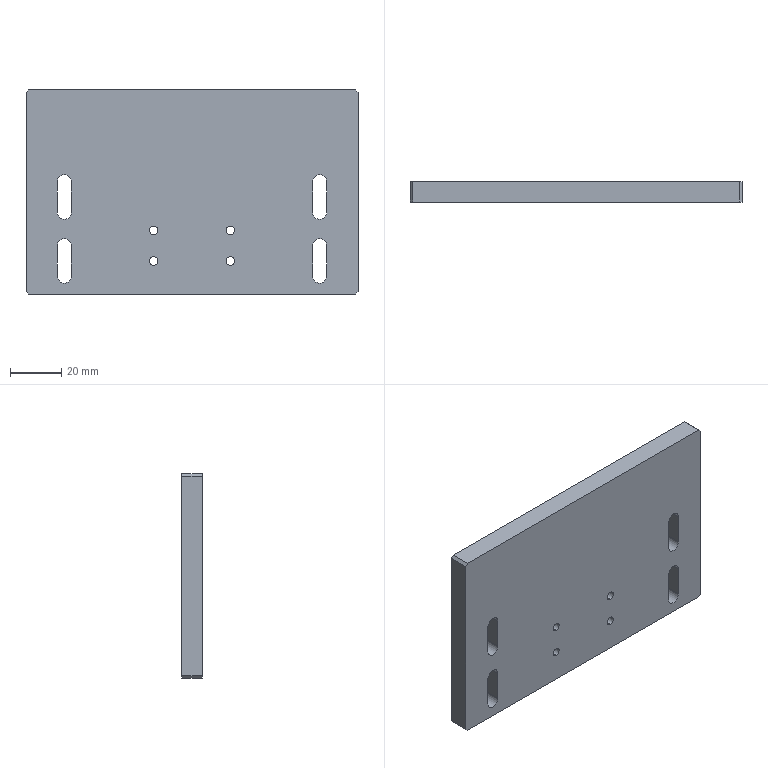Part | NX | features BREP 1 | 1 solid | 38 faces | box 130 x 8 x 80 mm | volume 80038 mm3 | cylinder 20 | plane 18 | commonest cylinder face diameters 5.5 x12 3.3 x8
STEP:
#1=CARTESIAN_POINT('',(15.,-4.,-16.65));
#2=VERTEX_POINT('',#1);
#3=CARTESIAN_POINT('',(15.,-4.,-13.35));
#4=VERTEX_POINT('',#3);
#5=CARTESIAN_POINT('',(15.,-4.,-15.));
#6=DIRECTION('',(0.,1.,0.));
#7=DIRECTION('',(0.,0.,1.));
#8=AXIS2_PLACEMENT_3D('',#5,#6,#7);
#9=CIRCLE('',#8,1.65);
#10=EDGE_CURVE('',#2,#4,#9,.T.);
#11=ORIENTED_EDGE('',*,*,#10,.F.);
#12=CARTESIAN_POINT('',(15.,4.,-16.65));
#13=VERTEX_POINT('',#12);
#14=CARTESIAN_POINT('',(15.,4.,-16.65));
#15=DIRECTION('',(0.,1.,0.));
#16=VECTOR('',#15,1000.);
#17=LINE('',#14,#16);
#18=EDGE_CURVE('',#13,#2,#17,.F.);
#19=ORIENTED_EDGE('',*,*,#18,.F.);
#20=CARTESIAN_POINT('',(15.,4.,-13.35));
#21=VERTEX_POINT('',#20);
#22=CARTESIAN_POINT('',(15.,4.,-15.));
#23=DIRECTION('',(0.,1.,0.));
#24=DIRECTION('',(0.,0.,1.));
#25=AXIS2_PLACEMENT_3D('',#22,#23,#24);
#26=CIRCLE('',#25,1.65);
#27=EDGE_CURVE('',#13,#21,#26,.T.);
#28=ORIENTED_EDGE('',*,*,#27,.T.);
#29=CARTESIAN_POINT('',(15.,4.,-13.35));
#30=DIRECTION('',(0.,1.,0.));
#31=VECTOR('',#30,1000.);
#32=LINE('',#29,#31);
#33=EDGE_CURVE('',#21,#4,#32,.F.);
#34=ORIENTED_EDGE('',*,*,#33,.T.);
#35=EDGE_LOOP('',(#11,#19,#28,#34));
#36=FACE_BOUND('',#35,.T.);
#37=CARTESIAN_POINT('',(15.,4.,-15.));
#38=DIRECTION('',(0.,1.,0.));
#39=DIRECTION('',(0.,0.,1.));
#40=AXIS2_PLACEMENT_3D('',#37,#38,#39);
#41=CYLINDRICAL_SURFACE('',#40,1.65);
#42=ADVANCED_FACE('',(#36),#41,.F.);
#43=CARTESIAN_POINT('',(15.,-4.,-28.65));
#44=VERTEX_POINT('',#43);
#45=CARTESIAN_POINT('',(15.,-4.,-25.35));
#46=VERTEX_POINT('',#45);
#47=CARTESIAN_POINT('',(15.,-4.,-27.));
#48=DIRECTION('',(0.,1.,0.));
#49=DIRECTION('',(0.,0.,1.));
#50=AXIS2_PLACEMENT_3D('',#47,#48,#49);
#51=CIRCLE('',#50,1.65);
#52=EDGE_CURVE('',#44,#46,#51,.T.);
#53=ORIENTED_EDGE('',*,*,#52,.F.);
#54=CARTESIAN_POINT('',(15.,4.,-28.65));
#55=VERTEX_POINT('',#54);
#56=CARTESIAN_POINT('',(15.,4.,-28.65));
#57=DIRECTION('',(0.,1.,0.));
#58=VECTOR('',#57,1000.);
#59=LINE('',#56,#58);
#60=EDGE_CURVE('',#55,#44,#59,.F.);
#61=ORIENTED_EDGE('',*,*,#60,.F.);
#62=CARTESIAN_POINT('',(15.,4.,-25.35));
#63=VERTEX_POINT('',#62);
#64=CARTESIAN_POINT('',(15.,4.,-27.));
#65=DIRECTION('',(0.,1.,0.));
#66=DIRECTION('',(0.,0.,1.));
#67=AXIS2_PLACEMENT_3D('',#64,#65,#66);
#68=CIRCLE('',#67,1.65);
#69=EDGE_CURVE('',#55,#63,#68,.T.);
#70=ORIENTED_EDGE('',*,*,#69,.T.);
#71=CARTESIAN_POINT('',(15.,4.,-25.35));
#72=DIRECTION('',(0.,1.,0.));
#73=VECTOR('',#72,1000.);
#74=LINE('',#71,#73);
#75=EDGE_CURVE('',#63,#46,#74,.F.);
#76=ORIENTED_EDGE('',*,*,#75,.T.);
#77=EDGE_LOOP('',(#53,#61,#70,#76));
#78=FACE_BOUND('',#77,.T.);
#79=CARTESIAN_POINT('',(15.,4.,-27.));
#80=DIRECTION('',(0.,1.,0.));
#81=DIRECTION('',(0.,0.,1.));
#82=AXIS2_PLACEMENT_3D('',#79,#80,#81);
#83=CYLINDRICAL_SURFACE('',#82,1.65);
#84=ADVANCED_FACE('',(#78),#83,.F.);
#85=CARTESIAN_POINT('',(-15.,-4.,-16.65));
#86=VERTEX_POINT('',#85);
#87=CARTESIAN_POINT('',(-15.,-4.,-13.35));
#88=VERTEX_POINT('',#87);
#89=CARTESIAN_POINT('',(-15.,-4.,-15.));
#90=DIRECTION('',(0.,1.,0.));
#91=DIRECTION('',(0.,0.,1.));
#92=AXIS2_PLACEMENT_3D('',#89,#90,#91);
#93=CIRCLE('',#92,1.65);
#94=EDGE_CURVE('',#86,#88,#93,.T.);
#95=ORIENTED_EDGE('',*,*,#94,.F.);
#96=CARTESIAN_POINT('',(-15.,4.,-16.65));
#97=VERTEX_POINT('',#96);
#98=CARTESIAN_POINT('',(-15.,4.,-16.65));
#99=DIRECTION('',(0.,1.,0.));
#100=VECTOR('',#99,1000.);
#101=LINE('',#98,#100);
#102=EDGE_CURVE('',#97,#86,#101,.F.);
#103=ORIENTED_EDGE('',*,*,#102,.F.);
#104=CARTESIAN_POINT('',(-15.,4.,-13.35));
#105=VERTEX_POINT('',#104);
#106=CARTESIAN_POINT('',(-15.,4.,-15.));
#107=DIRECTION('',(0.,1.,0.));
#108=DIRECTION('',(0.,0.,1.));
#109=AXIS2_PLACEMENT_3D('',#106,#107,#108);
#110=CIRCLE('',#109,1.65);
#111=EDGE_CURVE('',#97,#105,#110,.T.);
#112=ORIENTED_EDGE('',*,*,#111,.T.);
#113=CARTESIAN_POINT('',(-15.,4.,-13.35));
#114=DIRECTION('',(0.,1.,0.));
#115=VECTOR('',#114,1000.);
#116=LINE('',#113,#115);
#117=EDGE_CURVE('',#105,#88,#116,.F.);
#118=ORIENTED_EDGE('',*,*,#117,.T.);
#119=EDGE_LOOP('',(#95,#103,#112,#118));
#120=FACE_BOUND('',#119,.T.);
#121=CARTESIAN_POINT('',(-15.,4.,-15.));
#122=DIRECTION('',(0.,1.,0.));
#123=DIRECTION('',(0.,0.,1.));
#124=AXIS2_PLACEMENT_3D('',#121,#122,#123);
#125=CYLINDRICAL_SURFACE('',#124,1.65);
#126=ADVANCED_FACE('',(#120),#125,.F.);
#127=CARTESIAN_POINT('',(-15.,-4.,-28.65));
#128=VERTEX_POINT('',#127);
#129=CARTESIAN_POINT('',(-15.,-4.,-25.35));
#130=VERTEX_POINT('',#129);
#131=CARTESIAN_POINT('',(-15.,-4.,-27.));
#132=DIRECTION('',(0.,1.,0.));
#133=DIRECTION('',(0.,0.,1.));
#134=AXIS2_PLACEMENT_3D('',#131,#132,#133);
#135=CIRCLE('',#134,1.65);
#136=EDGE_CURVE('',#128,#130,#135,.T.);
#137=ORIENTED_EDGE('',*,*,#136,.F.);
#138=CARTESIAN_POINT('',(-15.,4.,-28.65));
#139=VERTEX_POINT('',#138);
#140=CARTESIAN_POINT('',(-15.,4.,-28.65));
#141=DIRECTION('',(0.,1.,0.));
#142=VECTOR('',#141,1000.);
#143=LINE('',#140,#142);
#144=EDGE_CURVE('',#139,#128,#143,.F.);
#145=ORIENTED_EDGE('',*,*,#144,.F.);
#146=CARTESIAN_POINT('',(-15.,4.,-25.35));
#147=VERTEX_POINT('',#146);
#148=CARTESIAN_POINT('',(-15.,4.,-27.));
#149=DIRECTION('',(0.,1.,0.));
#150=DIRECTION('',(0.,0.,1.));
#151=AXIS2_PLACEMENT_3D('',#148,#149,#150);
#152=CIRCLE('',#151,1.65);
#153=EDGE_CURVE('',#139,#147,#152,.T.);
#154=ORIENTED_EDGE('',*,*,#153,.T.);
#155=CARTESIAN_POINT('',(-15.,4.,-25.35));
#156=DIRECTION('',(0.,1.,0.));
#157=VECTOR('',#156,1000.);
#158=LINE('',#155,#157);
#159=EDGE_CURVE('',#147,#130,#158,.F.);
#160=ORIENTED_EDGE('',*,*,#159,.T.);
#161=EDGE_LOOP('',(#137,#145,#154,#160));
#162=FACE_BOUND('',#161,.T.);
#163=CARTESIAN_POINT('',(-15.,4.,-27.));
#164=DIRECTION('',(0.,1.,0.));
#165=DIRECTION('',(0.,0.,1.));
#166=AXIS2_PLACEMENT_3D('',#163,#164,#165);
#167=CYLINDRICAL_SURFACE('',#166,1.65);
#168=ADVANCED_FACE('',(#162),#167,.F.);
#169=CARTESIAN_POINT('',(52.75,-4.,4.));
#170=VERTEX_POINT('',#169);
#171=CARTESIAN_POINT('',(50.,-4.,6.75));
#172=VERTEX_POINT('',#171);
#173=CARTESIAN_POINT('',(50.,-4.,4.));
#174=DIRECTION('',(0.,-1.,0.));
#175=DIRECTION('',(0.,0.,1.));
#176=AXIS2_PLACEMENT_3D('',#173,#174,#175);
#177=CIRCLE('',#176,2.75);
#178=EDGE_CURVE('',#170,#172,#177,.T.);
#179=ORIENTED_EDGE('',*,*,#178,.T.);
#180=CARTESIAN_POINT('',(50.,4.,6.75));
#181=VERTEX_POINT('',#180);
#182=CARTESIAN_POINT('',(50.,-6.,6.75));
#183=DIRECTION('',(0.,1.,0.));
#184=VECTOR('',#183,1000.);
#185=LINE('',#182,#184);
#186=EDGE_CURVE('',#172,#181,#185,.T.);
#187=ORIENTED_EDGE('',*,*,#186,.T.);
#188=CARTESIAN_POINT('',(52.75,4.,4.));
#189=VERTEX_POINT('',#188);
#190=CARTESIAN_POINT('',(50.,4.,4.));
#191=DIRECTION('',(0.,-1.,0.));
#192=DIRECTION('',(0.,0.,1.));
#193=AXIS2_PLACEMENT_3D('',#190,#191,#192);
#194=CIRCLE('',#193,2.75);
#195=EDGE_CURVE('',#189,#181,#194,.T.);
#196=ORIENTED_EDGE('',*,*,#195,.F.);
#197=CARTESIAN_POINT('',(52.75,-6.,4.));
#198=DIRECTION('',(0.,1.,0.));
#199=VECTOR('',#198,1000.);
#200=LINE('',#197,#199);
#201=EDGE_CURVE('',#170,#189,#200,.T.);
#202=ORIENTED_EDGE('',*,*,#201,.F.);
#203=EDGE_LOOP('',(#179,#187,#196,#202));
#204=FACE_BOUND('',#203,.T.);
#205=CARTESIAN_POINT('',(50.,-6.,4.));
#206=DIRECTION('',(0.,1.,0.));
#207=DIRECTION('',(0.,0.,1.));
#208=AXIS2_PLACEMENT_3D('',#205,#206,#207);
#209=CYLINDRICAL_SURFACE('',#208,2.75);
#210=ADVANCED_FACE('',(#204),#209,.F.);
#211=CARTESIAN_POINT('',(52.75,-4.,-21.));
#212=VERTEX_POINT('',#211);
#213=CARTESIAN_POINT('',(50.,-4.,-18.25));
#214=VERTEX_POINT('',#213);
#215=CARTESIAN_POINT('',(50.,-4.,-21.));
#216=DIRECTION('',(0.,-1.,0.));
#217=DIRECTION('',(0.,0.,1.));
#218=AXIS2_PLACEMENT_3D('',#215,#216,#217);
#219=CIRCLE('',#218,2.75);
#220=EDGE_CURVE('',#212,#214,#219,.T.);
#221=ORIENTED_EDGE('',*,*,#220,.T.);
#222=CARTESIAN_POINT('',(50.,4.,-18.25));
#223=VERTEX_POINT('',#222);
#224=CARTESIAN_POINT('',(50.,-6.,-18.25));
#225=DIRECTION('',(0.,1.,0.));
#226=VECTOR('',#225,1000.);
#227=LINE('',#224,#226);
#228=EDGE_CURVE('',#214,#223,#227,.T.);
#229=ORIENTED_EDGE('',*,*,#228,.T.);
#230=CARTESIAN_POINT('',(52.75,4.,-21.));
#231=VERTEX_POINT('',#230);
#232=CARTESIAN_POINT('',(50.,4.,-21.));
#233=DIRECTION('',(0.,-1.,0.));
#234=DIRECTION('',(0.,0.,1.));
#235=AXIS2_PLACEMENT_3D('',#232,#233,#234);
#236=CIRCLE('',#235,2.75);
#237=EDGE_CURVE('',#231,#223,#236,.T.);
#238=ORIENTED_EDGE('',*,*,#237,.F.);
#239=CARTESIAN_POINT('',(52.75,-6.,-21.));
#240=DIRECTION('',(0.,1.,0.));
#241=VECTOR('',#240,1000.);
#242=LINE('',#239,#241);
#243=EDGE_CURVE('',#212,#231,#242,.T.);
#244=ORIENTED_EDGE('',*,*,#243,.F.);
#245=EDGE_LOOP('',(#221,#229,#238,#244));
#246=FACE_BOUND('',#245,.T.);
#247=CARTESIAN_POINT('',(50.,-6.,-21.));
#248=DIRECTION('',(0.,1.,0.));
#249=DIRECTION('',(0.,0.,1.));
#250=AXIS2_PLACEMENT_3D('',#247,#248,#249);
#251=CYLINDRICAL_SURFACE('',#250,2.75);
#252=ADVANCED_FACE('',(#246),#251,.F.);
#253=CARTESIAN_POINT('',(-50.,-4.,6.75));
#254=VERTEX_POINT('',#253);
#255=CARTESIAN_POINT('',(-47.25,-4.,4.));
#256=VERTEX_POINT('',#255);
#257=CARTESIAN_POINT('',(-50.,-4.,4.));
#258=DIRECTION('',(0.,1.,0.));
#259=DIRECTION('',(0.,0.,1.));
#260=AXIS2_PLACEMENT_3D('',#257,#258,#259);
#261=CIRCLE('',#260,2.75);
#262=EDGE_CURVE('',#254,#256,#261,.T.);
#263=ORIENTED_EDGE('',*,*,#262,.F.);
#264=CARTESIAN_POINT('',(-50.,4.,6.75));
#265=VERTEX_POINT('',#264);
#266=CARTESIAN_POINT('',(-50.,-6.,6.75));
#267=DIRECTION('',(0.,1.,0.));
#268=VECTOR('',#267,1000.);
#269=LINE('',#266,#268);
#270=EDGE_CURVE('',#254,#265,#269,.T.);
#271=ORIENTED_EDGE('',*,*,#270,.T.);
#272=CARTESIAN_POINT('',(-47.25,4.,4.));
#273=VERTEX_POINT('',#272);
#274=CARTESIAN_POINT('',(-50.,4.,4.));
#275=DIRECTION('',(0.,1.,0.));
#276=DIRECTION('',(0.,0.,1.));
#277=AXIS2_PLACEMENT_3D('',#274,#275,#276);
#278=CIRCLE('',#277,2.75);
#279=EDGE_CURVE('',#265,#273,#278,.T.);
#280=ORIENTED_EDGE('',*,*,#279,.T.);
#281=CARTESIAN_POINT('',(-47.25,-6.,4.));
#282=DIRECTION('',(0.,1.,0.));
#283=VECTOR('',#282,1000.);
#284=LINE('',#281,#283);
#285=EDGE_CURVE('',#256,#273,#284,.T.);
#286=ORIENTED_EDGE('',*,*,#285,.F.);
#287=EDGE_LOOP('',(#263,#271,#280,#286));
#288=FACE_BOUND('',#287,.T.);
#289=CARTESIAN_POINT('',(-50.,-6.,4.));
#290=DIRECTION('',(0.,1.,0.));
#291=DIRECTION('',(0.,0.,1.));
#292=AXIS2_PLACEMENT_3D('',#289,#290,#291);
#293=CYLINDRICAL_SURFACE('',#292,2.75);
#294=ADVANCED_FACE('',(#288),#293,.F.);
#295=CARTESIAN_POINT('',(-50.,-4.,-18.25));
#296=VERTEX_POINT('',#295);
#297=CARTESIAN_POINT('',(-47.25,-4.,-21.));
#298=VERTEX_POINT('',#297);
#299=CARTESIAN_POINT('',(-50.,-4.,-21.));
#300=DIRECTION('',(0.,1.,0.));
#301=DIRECTION('',(0.,0.,1.));
#302=AXIS2_PLACEMENT_3D('',#299,#300,#301);
#303=CIRCLE('',#302,2.75);
#304=EDGE_CURVE('',#296,#298,#303,.T.);
#305=ORIENTED_EDGE('',*,*,#304,.F.);
#306=CARTESIAN_POINT('',(-50.,4.,-18.25));
#307=VERTEX_POINT('',#306);
#308=CARTESIAN_POINT('',(-50.,-6.,-18.25));
#309=DIRECTION('',(0.,1.,0.));
#310=VECTOR('',#309,1000.);
#311=LINE('',#308,#310);
#312=EDGE_CURVE('',#296,#307,#311,.T.);
#313=ORIENTED_EDGE('',*,*,#312,.T.);
#314=CARTESIAN_POINT('',(-47.25,4.,-21.));
#315=VERTEX_POINT('',#314);
#316=CARTESIAN_POINT('',(-50.,4.,-21.));
#317=DIRECTION('',(0.,1.,0.));
#318=DIRECTION('',(0.,0.,1.));
#319=AXIS2_PLACEMENT_3D('',#316,#317,#318);
#320=CIRCLE('',#319,2.75);
#321=EDGE_CURVE('',#307,#315,#320,.T.);
#322=ORIENTED_EDGE('',*,*,#321,.T.);
#323=CARTESIAN_POINT('',(-47.25,-6.,-21.));
#324=DIRECTION('',(0.,1.,0.));
#325=VECTOR('',#324,1000.);
#326=LINE('',#323,#325);
#327=EDGE_CURVE('',#298,#315,#326,.T.);
#328=ORIENTED_EDGE('',*,*,#327,.F.);
#329=EDGE_LOOP('',(#305,#313,#322,#328));
#330=FACE_BOUND('',#329,.T.);
#331=CARTESIAN_POINT('',(-50.,-6.,-21.));
#332=DIRECTION('',(0.,1.,0.));
#333=DIRECTION('',(0.,0.,1.));
#334=AXIS2_PLACEMENT_3D('',#331,#332,#333);
#335=CYLINDRICAL_SURFACE('',#334,2.75);
#336=ADVANCED_FACE('',(#330),#335,.F.);
#337=CARTESIAN_POINT('',(64.,4.,-40.));
#338=VERTEX_POINT('',#337);
#339=CARTESIAN_POINT('',(-64.,4.,-40.));
#340=VERTEX_POINT('',#339);
#341=CARTESIAN_POINT('',(-65.,4.,-40.));
#342=DIRECTION('',(-1.,0.,0.));
#343=VECTOR('',#342,1000.);
#344=LINE('',#341,#343);
#345=EDGE_CURVE('',#338,#340,#344,.T.);
#346=ORIENTED_EDGE('',*,*,#345,.T.);
#347=CARTESIAN_POINT('',(-65.,4.,-39.));
#348=VERTEX_POINT('',#347);
#349=CARTESIAN_POINT('',(-52.,4.,-52.));
#350=DIRECTION('',(-0.7071,0.,0.7071));
#351=VECTOR('',#350,1000.);
#352=LINE('',#349,#351);
#353=EDGE_CURVE('',#340,#348,#352,.T.);
#354=ORIENTED_EDGE('',*,*,#353,.T.);
#355=CARTESIAN_POINT('',(-65.,4.,39.));
#356=VERTEX_POINT('',#355);
#357=CARTESIAN_POINT('',(-65.,4.,-40.));
#358=DIRECTION('',(0.,0.,1.));
#359=VECTOR('',#358,1000.);
#360=LINE('',#357,#359);
#361=EDGE_CURVE('',#348,#356,#360,.T.);
#362=ORIENTED_EDGE('',*,*,#361,.T.);
#363=CARTESIAN_POINT('',(-64.,4.,40.));
#364=VERTEX_POINT('',#363);
#365=CARTESIAN_POINT('',(-52.,4.,52.));
#366=DIRECTION('',(0.7071,0.,0.7071));
#367=VECTOR('',#366,1000.);
#368=LINE('',#365,#367);
#369=EDGE_CURVE('',#356,#364,#368,.T.);
#370=ORIENTED_EDGE('',*,*,#369,.T.);
#371=CARTESIAN_POINT('',(64.,4.,40.));
#372=VERTEX_POINT('',#371);
#373=CARTESIAN_POINT('',(-65.,4.,40.));
#374=DIRECTION('',(1.,0.,0.));
#375=VECTOR('',#374,1000.);
#376=LINE('',#373,#375);
#377=EDGE_CURVE('',#364,#372,#376,.T.);
#378=ORIENTED_EDGE('',*,*,#377,.T.);
#379=CARTESIAN_POINT('',(65.,4.,39.));
#380=VERTEX_POINT('',#379);
#381=CARTESIAN_POINT('',(52.,4.,52.));
#382=DIRECTION('',(0.7071,0.,-0.7071));
#383=VECTOR('',#382,1000.);
#384=LINE('',#381,#383);
#385=EDGE_CURVE('',#372,#380,#384,.T.);
#386=ORIENTED_EDGE('',*,*,#385,.T.);
#387=CARTESIAN_POINT('',(65.,4.,-39.));
#388=VERTEX_POINT('',#387);
#389=CARTESIAN_POINT('',(65.,4.,-40.));
#390=DIRECTION('',(0.,0.,-1.));
#391=VECTOR('',#390,1000.);
#392=LINE('',#389,#391);
#393=EDGE_CURVE('',#380,#388,#392,.T.);
#394=ORIENTED_EDGE('',*,*,#393,.T.);
#395=CARTESIAN_POINT('',(52.,4.,-52.));
#396=DIRECTION('',(-0.7071,0.,-0.7071));
#397=VECTOR('',#396,1000.);
#398=LINE('',#395,#397);
#399=EDGE_CURVE('',#388,#338,#398,.T.);
#400=ORIENTED_EDGE('',*,*,#399,.T.);
#401=EDGE_LOOP('',(#346,#354,#362,#370,#378,#386,#394,#400));
#402=FACE_BOUND('',#401,.T.);
#403=CARTESIAN_POINT('',(15.,4.,-15.));
#404=DIRECTION('',(0.,1.,0.));
#405=DIRECTION('',(0.,0.,1.));
#406=AXIS2_PLACEMENT_3D('',#403,#404,#405);
#407=CIRCLE('',#406,1.65);
#408=EDGE_CURVE('',#21,#13,#407,.T.);
#409=ORIENTED_EDGE('',*,*,#408,.F.);
#410=ORIENTED_EDGE('',*,*,#27,.F.);
#411=EDGE_LOOP('',(#409,#410));
#412=FACE_BOUND('',#411,.T.);
#413=CARTESIAN_POINT('',(15.,4.,-27.));
#414=DIRECTION('',(0.,1.,0.));
#415=DIRECTION('',(0.,0.,1.));
#416=AXIS2_PLACEMENT_3D('',#413,#414,#415);
#417=CIRCLE('',#416,1.65);
#418=EDGE_CURVE('',#63,#55,#417,.T.);
#419=ORIENTED_EDGE('',*,*,#418,.F.);
#420=ORIENTED_EDGE('',*,*,#69,.F.);
#421=EDGE_LOOP('',(#419,#420));
#422=FACE_BOUND('',#421,.T.);
#423=CARTESIAN_POINT('',(-15.,4.,-15.));
#424=DIRECTION('',(0.,1.,0.));
#425=DIRECTION('',(0.,0.,1.));
#426=AXIS2_PLACEMENT_3D('',#423,#424,#425);
#427=CIRCLE('',#426,1.65);
#428=EDGE_CURVE('',#105,#97,#427,.T.);
#429=ORIENTED_EDGE('',*,*,#428,.F.);
#430=ORIENTED_EDGE('',*,*,#111,.F.);
#431=EDGE_LOOP('',(#429,#430));
#432=FACE_BOUND('',#431,.T.);
#433=CARTESIAN_POINT('',(-15.,4.,-27.));
#434=DIRECTION('',(0.,1.,0.));
#435=DIRECTION('',(0.,0.,1.));
#436=AXIS2_PLACEMENT_3D('',#433,#434,#435);
#437=CIRCLE('',#436,1.65);
#438=EDGE_CURVE('',#147,#139,#437,.T.);
#439=ORIENTED_EDGE('',*,*,#438,.F.);
#440=ORIENTED_EDGE('',*,*,#153,.F.);
#441=EDGE_LOOP('',(#439,#440));
#442=FACE_BOUND('',#441,.T.);
#443=CARTESIAN_POINT('',(47.25,4.,-21.));
#444=VERTEX_POINT('',#443);
#445=CARTESIAN_POINT('',(47.25,4.,-33.));
#446=VERTEX_POINT('',#445);
#447=CARTESIAN_POINT('',(47.25,4.,-33.));
#448=DIRECTION('',(0.,0.,-1.));
#449=VECTOR('',#448,1000.);
#450=LINE('',#447,#449);
#451=EDGE_CURVE('',#444,#446,#450,.T.);
#452=ORIENTED_EDGE('',*,*,#451,.T.);
#453=CARTESIAN_POINT('',(52.75,4.,-33.));
#454=VERTEX_POINT('',#453);
#455=CARTESIAN_POINT('',(50.,4.,-33.));
#456=DIRECTION('',(0.,-1.,0.));
#457=DIRECTION('',(0.,0.,1.));
#458=AXIS2_PLACEMENT_3D('',#455,#456,#457);
#459=CIRCLE('',#458,2.75);
#460=EDGE_CURVE('',#446,#454,#459,.T.);
#461=ORIENTED_EDGE('',*,*,#460,.T.);
#462=CARTESIAN_POINT('',(52.75,4.,-33.));
#463=DIRECTION('',(0.,0.,1.));
#464=VECTOR('',#463,1000.);
#465=LINE('',#462,#464);
#466=EDGE_CURVE('',#454,#231,#465,.T.);
#467=ORIENTED_EDGE('',*,*,#466,.T.);
#468=ORIENTED_EDGE('',*,*,#237,.T.);
#469=CARTESIAN_POINT('',(50.,4.,-21.));
#470=DIRECTION('',(0.,-1.,0.));
#471=DIRECTION('',(0.,0.,1.));
#472=AXIS2_PLACEMENT_3D('',#469,#470,#471);
#473=CIRCLE('',#472,2.75);
#474=EDGE_CURVE('',#223,#444,#473,.T.);
#475=ORIENTED_EDGE('',*,*,#474,.T.);
#476=EDGE_LOOP('',(#452,#461,#467,#468,#475));
#477=FACE_BOUND('',#476,.T.);
#478=CARTESIAN_POINT('',(-47.25,4.,-8.));
#479=VERTEX_POINT('',#478);
#480=CARTESIAN_POINT('',(-52.75,4.,-8.));
#481=VERTEX_POINT('',#480);
#482=CARTESIAN_POINT('',(-50.,4.,-8.));
#483=DIRECTION('',(0.,1.,0.));
#484=DIRECTION('',(0.,0.,1.));
#485=AXIS2_PLACEMENT_3D('',#482,#483,#484);
#486=CIRCLE('',#485,2.75);
#487=EDGE_CURVE('',#479,#481,#486,.T.);
#488=ORIENTED_EDGE('',*,*,#487,.F.);
#489=CARTESIAN_POINT('',(-47.25,4.,-8.));
#490=DIRECTION('',(0.,0.,-1.));
#491=VECTOR('',#490,1000.);
#492=LINE('',#489,#491);
#493=EDGE_CURVE('',#273,#479,#492,.T.);
#494=ORIENTED_EDGE('',*,*,#493,.F.);
#495=ORIENTED_EDGE('',*,*,#279,.F.);
#496=CARTESIAN_POINT('',(-52.75,4.,4.));
#497=VERTEX_POINT('',#496);
#498=CARTESIAN_POINT('',(-50.,4.,4.));
#499=DIRECTION('',(0.,1.,0.));
#500=DIRECTION('',(0.,0.,1.));
#501=AXIS2_PLACEMENT_3D('',#498,#499,#500);
#502=CIRCLE('',#501,2.75);
#503=EDGE_CURVE('',#497,#265,#502,.T.);
#504=ORIENTED_EDGE('',*,*,#503,.F.);
#505=CARTESIAN_POINT('',(-52.75,4.,-8.));
#506=DIRECTION('',(0.,0.,1.));
#507=VECTOR('',#506,1000.);
#508=LINE('',#505,#507);
#509=EDGE_CURVE('',#481,#497,#508,.T.);
#510=ORIENTED_EDGE('',*,*,#509,.F.);
#511=EDGE_LOOP('',(#488,#494,#495,#504,#510));
#512=FACE_BOUND('',#511,.T.);
#513=CARTESIAN_POINT('',(-47.25,4.,-33.));
#514=VERTEX_POINT('',#513);
#515=CARTESIAN_POINT('',(-52.75,4.,-33.));
#516=VERTEX_POINT('',#515);
#517=CARTESIAN_POINT('',(-50.,4.,-33.));
#518=DIRECTION('',(0.,1.,0.));
#519=DIRECTION('',(0.,0.,1.));
#520=AXIS2_PLACEMENT_3D('',#517,#518,#519);
#521=CIRCLE('',#520,2.75);
#522=EDGE_CURVE('',#514,#516,#521,.T.);
#523=ORIENTED_EDGE('',*,*,#522,.F.);
#524=CARTESIAN_POINT('',(-47.25,4.,-33.));
#525=DIRECTION('',(0.,0.,-1.));
#526=VECTOR('',#525,1000.);
#527=LINE('',#524,#526);
#528=EDGE_CURVE('',#315,#514,#527,.T.);
#529=ORIENTED_EDGE('',*,*,#528,.F.);
#530=ORIENTED_EDGE('',*,*,#321,.F.);
#531=CARTESIAN_POINT('',(-52.75,4.,-21.));
#532=VERTEX_POINT('',#531);
#533=CARTESIAN_POINT('',(-50.,4.,-21.));
#534=DIRECTION('',(0.,1.,0.));
#535=DIRECTION('',(0.,0.,1.));
#536=AXIS2_PLACEMENT_3D('',#533,#534,#535);
#537=CIRCLE('',#536,2.75);
#538=EDGE_CURVE('',#532,#307,#537,.T.);
#539=ORIENTED_EDGE('',*,*,#538,.F.);
#540=CARTESIAN_POINT('',(-52.75,4.,-33.));
#541=DIRECTION('',(0.,0.,1.));
#542=VECTOR('',#541,1000.);
#543=LINE('',#540,#542);
#544=EDGE_CURVE('',#516,#532,#543,.T.);
#545=ORIENTED_EDGE('',*,*,#544,.F.);
#546=EDGE_LOOP('',(#523,#529,#530,#539,#545));
#547=FACE_BOUND('',#546,.T.);
#548=CARTESIAN_POINT('',(47.25,4.,4.));
#549=VERTEX_POINT('',#548);
#550=CARTESIAN_POINT('',(47.25,4.,-8.));
#551=VERTEX_POINT('',#550);
#552=CARTESIAN_POINT('',(47.25,4.,-8.));
#553=DIRECTION('',(0.,0.,-1.));
#554=VECTOR('',#553,1000.);
#555=LINE('',#552,#554);
#556=EDGE_CURVE('',#549,#551,#555,.T.);
#557=ORIENTED_EDGE('',*,*,#556,.T.);
#558=CARTESIAN_POINT('',(52.75,4.,-8.));
#559=VERTEX_POINT('',#558);
#560=CARTESIAN_POINT('',(50.,4.,-8.));
#561=DIRECTION('',(0.,-1.,0.));
#562=DIRECTION('',(0.,0.,1.));
#563=AXIS2_PLACEMENT_3D('',#560,#561,#562);
#564=CIRCLE('',#563,2.75);
#565=EDGE_CURVE('',#551,#559,#564,.T.);
#566=ORIENTED_EDGE('',*,*,#565,.T.);
#567=CARTESIAN_POINT('',(52.75,4.,-8.));
#568=DIRECTION('',(0.,0.,1.));
#569=VECTOR('',#568,1000.);
#570=LINE('',#567,#569);
#571=EDGE_CURVE('',#559,#189,#570,.T.);
#572=ORIENTED_EDGE('',*,*,#571,.T.);
#573=ORIENTED_EDGE('',*,*,#195,.T.);
#574=CARTESIAN_POINT('',(50.,4.,4.));
#575=DIRECTION('',(0.,-1.,0.));
#576=DIRECTION('',(0.,0.,1.));
#577=AXIS2_PLACEMENT_3D('',#574,#575,#576);
#578=CIRCLE('',#577,2.75);
#579=EDGE_CURVE('',#181,#549,#578,.T.);
#580=ORIENTED_EDGE('',*,*,#579,.T.);
#581=EDGE_LOOP('',(#557,#566,#572,#573,#580));
#582=FACE_BOUND('',#581,.T.);
#583=CARTESIAN_POINT('',(0.,4.,0.));
#584=DIRECTION('',(0.,1.,0.));
#585=DIRECTION('',(1.,0.,0.));
#586=AXIS2_PLACEMENT_3D('',#583,#584,#585);
#587=PLANE('',#586);
#588=ADVANCED_FACE('',(#402,#412,#422,#432,#442,#477,#512,#547,#582),#587,.T.);
#589=CARTESIAN_POINT('',(-65.,-4.,-39.));
#590=VERTEX_POINT('',#589);
#591=CARTESIAN_POINT('',(-65.,-4.,39.));
#592=VERTEX_POINT('',#591);
#593=CARTESIAN_POINT('',(-65.,-4.,-40.));
#594=DIRECTION('',(0.,0.,1.));
#595=VECTOR('',#594,1000.);
#596=LINE('',#593,#595);
#597=EDGE_CURVE('',#590,#592,#596,.T.);
#598=ORIENTED_EDGE('',*,*,#597,.F.);
#599=CARTESIAN_POINT('',(-64.,-4.,-40.));
#600=VERTEX_POINT('',#599);
#601=CARTESIAN_POINT('',(-65.,-4.,-39.));
#602=DIRECTION('',(0.7071,0.,-0.7071));
#603=VECTOR('',#602,1000.);
#604=LINE('',#601,#603);
#605=EDGE_CURVE('',#590,#600,#604,.T.);
#606=ORIENTED_EDGE('',*,*,#605,.T.);
#607=CARTESIAN_POINT('',(64.,-4.,-40.));
#608=VERTEX_POINT('',#607);
#609=CARTESIAN_POINT('',(-65.,-4.,-40.));
#610=DIRECTION('',(-1.,0.,0.));
#611=VECTOR('',#610,1000.);
#612=LINE('',#609,#611);
#613=EDGE_CURVE('',#608,#600,#612,.T.);
#614=ORIENTED_EDGE('',*,*,#613,.F.);
#615=CARTESIAN_POINT('',(65.,-4.,-39.));
#616=VERTEX_POINT('',#615);
#617=CARTESIAN_POINT('',(64.,-4.,-40.));
#618=DIRECTION('',(0.7071,0.,0.7071));
#619=VECTOR('',#618,1000.);
#620=LINE('',#617,#619);
#621=EDGE_CURVE('',#608,#616,#620,.T.);
#622=ORIENTED_EDGE('',*,*,#621,.T.);
#623=CARTESIAN_POINT('',(65.,-4.,39.));
#624=VERTEX_POINT('',#623);
#625=CARTESIAN_POINT('',(65.,-4.,-40.));
#626=DIRECTION('',(0.,0.,-1.));
#627=VECTOR('',#626,1000.);
#628=LINE('',#625,#627);
#629=EDGE_CURVE('',#624,#616,#628,.T.);
#630=ORIENTED_EDGE('',*,*,#629,.F.);
#631=CARTESIAN_POINT('',(64.,-4.,40.));
#632=VERTEX_POINT('',#631);
#633=CARTESIAN_POINT('',(65.,-4.,39.));
#634=DIRECTION('',(-0.7071,0.,0.7071));
#635=VECTOR('',#634,1000.);
#636=LINE('',#633,#635);
#637=EDGE_CURVE('',#624,#632,#636,.T.);
#638=ORIENTED_EDGE('',*,*,#637,.T.);
#639=CARTESIAN_POINT('',(-64.,-4.,40.));
#640=VERTEX_POINT('',#639);
#641=CARTESIAN_POINT('',(-65.,-4.,40.));
#642=DIRECTION('',(1.,0.,0.));
#643=VECTOR('',#642,1000.);
#644=LINE('',#641,#643);
#645=EDGE_CURVE('',#640,#632,#644,.T.);
#646=ORIENTED_EDGE('',*,*,#645,.F.);
#647=CARTESIAN_POINT('',(-64.,-4.,40.));
#648=DIRECTION('',(-0.7071,0.,-0.7071));
#649=VECTOR('',#648,1000.);
#650=LINE('',#647,#649);
#651=EDGE_CURVE('',#640,#592,#650,.T.);
#652=ORIENTED_EDGE('',*,*,#651,.T.);
#653=EDGE_LOOP('',(#598,#606,#614,#622,#630,#638,#646,#652));
#654=FACE_BOUND('',#653,.T.);
#655=CARTESIAN_POINT('',(15.,-4.,-15.));
#656=DIRECTION('',(0.,1.,0.));
#657=DIRECTION('',(0.,0.,1.));
#658=AXIS2_PLACEMENT_3D('',#655,#656,#657);
#659=CIRCLE('',#658,1.65);
#660=EDGE_CURVE('',#4,#2,#659,.T.);
#661=ORIENTED_EDGE('',*,*,#660,.T.);
#662=ORIENTED_EDGE('',*,*,#10,.T.);
#663=EDGE_LOOP('',(#661,#662));
#664=FACE_BOUND('',#663,.T.);
#665=CARTESIAN_POINT('',(15.,-4.,-27.));
#666=DIRECTION('',(0.,1.,0.));
#667=DIRECTION('',(0.,0.,1.));
#668=AXIS2_PLACEMENT_3D('',#665,#666,#667);
#669=CIRCLE('',#668,1.65);
#670=EDGE_CURVE('',#46,#44,#669,.T.);
#671=ORIENTED_EDGE('',*,*,#670,.T.);
#672=ORIENTED_EDGE('',*,*,#52,.T.);
#673=EDGE_LOOP('',(#671,#672));
#674=FACE_BOUND('',#673,.T.);
#675=CARTESIAN_POINT('',(-15.,-4.,-15.));
#676=DIRECTION('',(0.,1.,0.));
#677=DIRECTION('',(0.,0.,1.));
#678=AXIS2_PLACEMENT_3D('',#675,#676,#677);
#679=CIRCLE('',#678,1.65);
#680=EDGE_CURVE('',#88,#86,#679,.T.);
#681=ORIENTED_EDGE('',*,*,#680,.T.);
#682=ORIENTED_EDGE('',*,*,#94,.T.);
#683=EDGE_LOOP('',(#681,#682));
#684=FACE_BOUND('',#683,.T.);
#685=CARTESIAN_POINT('',(-15.,-4.,-27.));
#686=DIRECTION('',(0.,1.,0.));
#687=DIRECTION('',(0.,0.,1.));
#688=AXIS2_PLACEMENT_3D('',#685,#686,#687);
#689=CIRCLE('',#688,1.65);
#690=EDGE_CURVE('',#130,#128,#689,.T.);
#691=ORIENTED_EDGE('',*,*,#690,.T.);
#692=ORIENTED_EDGE('',*,*,#136,.T.);
#693=EDGE_LOOP('',(#691,#692));
#694=FACE_BOUND('',#693,.T.);
#695=CARTESIAN_POINT('',(47.25,-4.,-33.));
#696=VERTEX_POINT('',#695);
#697=CARTESIAN_POINT('',(52.75,-4.,-33.));
#698=VERTEX_POINT('',#697);
#699=CARTESIAN_POINT('',(50.,-4.,-33.));
#700=DIRECTION('',(0.,-1.,0.));
#701=DIRECTION('',(0.,0.,1.));
#702=AXIS2_PLACEMENT_3D('',#699,#700,#701);
#703=CIRCLE('',#702,2.75);
#704=EDGE_CURVE('',#696,#698,#703,.T.);
#705=ORIENTED_EDGE('',*,*,#704,.F.);
#706=CARTESIAN_POINT('',(47.25,-4.,-21.));
#707=VERTEX_POINT('',#706);
#708=CARTESIAN_POINT('',(47.25,-4.,0.));
#709=DIRECTION('',(0.,0.,-1.));
#710=VECTOR('',#709,1000.);
#711=LINE('',#708,#710);
#712=EDGE_CURVE('',#707,#696,#711,.T.);
#713=ORIENTED_EDGE('',*,*,#712,.F.);
#714=CARTESIAN_POINT('',(50.,-4.,-21.));
#715=DIRECTION('',(0.,-1.,0.));
#716=DIRECTION('',(0.,0.,1.));
#717=AXIS2_PLACEMENT_3D('',#714,#715,#716);
#718=CIRCLE('',#717,2.75);
#719=EDGE_CURVE('',#214,#707,#718,.T.);
#720=ORIENTED_EDGE('',*,*,#719,.F.);
#721=ORIENTED_EDGE('',*,*,#220,.F.);
#722=CARTESIAN_POINT('',(52.75,-4.,0.));
#723=DIRECTION('',(0.,0.,1.));
#724=VECTOR('',#723,1000.);
#725=LINE('',#722,#724);
#726=EDGE_CURVE('',#698,#212,#725,.T.);
#727=ORIENTED_EDGE('',*,*,#726,.F.);
#728=EDGE_LOOP('',(#705,#713,#720,#721,#727));
#729=FACE_BOUND('',#728,.T.);
#730=CARTESIAN_POINT('',(-47.25,-4.,-8.));
#731=VERTEX_POINT('',#730);
#732=CARTESIAN_POINT('',(-47.25,-4.,0.));
#733=DIRECTION('',(0.,0.,-1.));
#734=VECTOR('',#733,1000.);
#735=LINE('',#732,#734);
#736=EDGE_CURVE('',#256,#731,#735,.T.);
#737=ORIENTED_EDGE('',*,*,#736,.T.);
#738=CARTESIAN_POINT('',(-52.75,-4.,-8.));
#739=VERTEX_POINT('',#738);
#740=CARTESIAN_POINT('',(-50.,-4.,-8.));
#741=DIRECTION('',(0.,1.,0.));
#742=DIRECTION('',(0.,0.,1.));
#743=AXIS2_PLACEMENT_3D('',#740,#741,#742);
#744=CIRCLE('',#743,2.75);
#745=EDGE_CURVE('',#731,#739,#744,.T.);
#746=ORIENTED_EDGE('',*,*,#745,.T.);
#747=CARTESIAN_POINT('',(-52.75,-4.,4.));
#748=VERTEX_POINT('',#747);
#749=CARTESIAN_POINT('',(-52.75,-4.,0.));
#750=DIRECTION('',(0.,0.,1.));
#751=VECTOR('',#750,1000.);
#752=LINE('',#749,#751);
#753=EDGE_CURVE('',#739,#748,#752,.T.);
#754=ORIENTED_EDGE('',*,*,#753,.T.);
#755=CARTESIAN_POINT('',(-50.,-4.,4.));
#756=DIRECTION('',(0.,1.,0.));
#757=DIRECTION('',(0.,0.,1.));
#758=AXIS2_PLACEMENT_3D('',#755,#756,#757);
#759=CIRCLE('',#758,2.75);
#760=EDGE_CURVE('',#748,#254,#759,.T.);
#761=ORIENTED_EDGE('',*,*,#760,.T.);
#762=ORIENTED_EDGE('',*,*,#262,.T.);
#763=EDGE_LOOP('',(#737,#746,#754,#761,#762));
#764=FACE_BOUND('',#763,.T.);
#765=CARTESIAN_POINT('',(-47.25,-4.,-33.));
#766=VERTEX_POINT('',#765);
#767=CARTESIAN_POINT('',(-47.25,-4.,0.));
#768=DIRECTION('',(0.,0.,-1.));
#769=VECTOR('',#768,1000.);
#770=LINE('',#767,#769);
#771=EDGE_CURVE('',#298,#766,#770,.T.);
#772=ORIENTED_EDGE('',*,*,#771,.T.);
#773=CARTESIAN_POINT('',(-52.75,-4.,-33.));
#774=VERTEX_POINT('',#773);
#775=CARTESIAN_POINT('',(-50.,-4.,-33.));
#776=DIRECTION('',(0.,1.,0.));
#777=DIRECTION('',(0.,0.,1.));
#778=AXIS2_PLACEMENT_3D('',#775,#776,#777);
#779=CIRCLE('',#778,2.75);
#780=EDGE_CURVE('',#766,#774,#779,.T.);
#781=ORIENTED_EDGE('',*,*,#780,.T.);
#782=CARTESIAN_POINT('',(-52.75,-4.,-21.));
#783=VERTEX_POINT('',#782);
#784=CARTESIAN_POINT('',(-52.75,-4.,0.));
#785=DIRECTION('',(0.,0.,1.));
#786=VECTOR('',#785,1000.);
#787=LINE('',#784,#786);
#788=EDGE_CURVE('',#774,#783,#787,.T.);
#789=ORIENTED_EDGE('',*,*,#788,.T.);
#790=CARTESIAN_POINT('',(-50.,-4.,-21.));
#791=DIRECTION('',(0.,1.,0.));
#792=DIRECTION('',(0.,0.,1.));
#793=AXIS2_PLACEMENT_3D('',#790,#791,#792);
#794=CIRCLE('',#793,2.75);
#795=EDGE_CURVE('',#783,#296,#794,.T.);
#796=ORIENTED_EDGE('',*,*,#795,.T.);
#797=ORIENTED_EDGE('',*,*,#304,.T.);
#798=EDGE_LOOP('',(#772,#781,#789,#796,#797));
#799=FACE_BOUND('',#798,.T.);
#800=CARTESIAN_POINT('',(47.25,-4.,-8.));
#801=VERTEX_POINT('',#800);
#802=CARTESIAN_POINT('',(52.75,-4.,-8.));
#803=VERTEX_POINT('',#802);
#804=CARTESIAN_POINT('',(50.,-4.,-8.));
#805=DIRECTION('',(0.,-1.,0.));
#806=DIRECTION('',(0.,0.,1.));
#807=AXIS2_PLACEMENT_3D('',#804,#805,#806);
#808=CIRCLE('',#807,2.75);
#809=EDGE_CURVE('',#801,#803,#808,.T.);
#810=ORIENTED_EDGE('',*,*,#809,.F.);
#811=CARTESIAN_POINT('',(47.25,-4.,4.));
#812=VERTEX_POINT('',#811);
#813=CARTESIAN_POINT('',(47.25,-4.,0.));
#814=DIRECTION('',(0.,0.,-1.));
#815=VECTOR('',#814,1000.);
#816=LINE('',#813,#815);
#817=EDGE_CURVE('',#812,#801,#816,.T.);
#818=ORIENTED_EDGE('',*,*,#817,.F.);
#819=CARTESIAN_POINT('',(50.,-4.,4.));
#820=DIRECTION('',(0.,-1.,0.));
#821=DIRECTION('',(0.,0.,1.));
#822=AXIS2_PLACEMENT_3D('',#819,#820,#821);
#823=CIRCLE('',#822,2.75);
#824=EDGE_CURVE('',#172,#812,#823,.T.);
#825=ORIENTED_EDGE('',*,*,#824,.F.);
#826=ORIENTED_EDGE('',*,*,#178,.F.);
#827=CARTESIAN_POINT('',(52.75,-4.,0.));
#828=DIRECTION('',(0.,0.,1.));
#829=VECTOR('',#828,1000.);
#830=LINE('',#827,#829);
#831=EDGE_CURVE('',#803,#170,#830,.T.);
#832=ORIENTED_EDGE('',*,*,#831,.F.);
#833=EDGE_LOOP('',(#810,#818,#825,#826,#832));
#834=FACE_BOUND('',#833,.T.);
#835=CARTESIAN_POINT('',(0.,-4.,0.));
#836=DIRECTION('',(0.,1.,0.));
#837=DIRECTION('',(1.,0.,0.));
#838=AXIS2_PLACEMENT_3D('',#835,#836,#837);
#839=PLANE('',#838);
#840=ADVANCED_FACE('',(#654,#664,#674,#684,#694,#729,#764,#799,#834),#839,.F.);
#841=ORIENTED_EDGE('',*,*,#629,.T.);
#842=CARTESIAN_POINT('',(65.,4.,-39.));
#843=DIRECTION('',(0.,1.,0.));
#844=VECTOR('',#843,1000.);
#845=LINE('',#842,#844);
#846=EDGE_CURVE('',#616,#388,#845,.T.);
#847=ORIENTED_EDGE('',*,*,#846,.T.);
#848=ORIENTED_EDGE('',*,*,#393,.F.);
#849=CARTESIAN_POINT('',(65.,4.,39.));
#850=DIRECTION('',(0.,-1.,0.));
#851=VECTOR('',#850,1000.);
#852=LINE('',#849,#851);
#853=EDGE_CURVE('',#380,#624,#852,.T.);
#854=ORIENTED_EDGE('',*,*,#853,.T.);
#855=EDGE_LOOP('',(#841,#847,#848,#854));
#856=FACE_BOUND('',#855,.T.);
#857=CARTESIAN_POINT('',(65.,4.,-40.));
#858=DIRECTION('',(-1.,0.,0.));
#859=DIRECTION('',(0.,0.,1.));
#860=AXIS2_PLACEMENT_3D('',#857,#858,#859);
#861=PLANE('',#860);
#862=ADVANCED_FACE('',(#856),#861,.F.);
#863=ORIENTED_EDGE('',*,*,#613,.T.);
#864=CARTESIAN_POINT('',(-64.,4.,-40.));
#865=DIRECTION('',(0.,1.,0.));
#866=VECTOR('',#865,1000.);
#867=LINE('',#864,#866);
#868=EDGE_CURVE('',#600,#340,#867,.T.);
#869=ORIENTED_EDGE('',*,*,#868,.T.);
#870=ORIENTED_EDGE('',*,*,#345,.F.);
#871=CARTESIAN_POINT('',(64.,4.,-40.));
#872=DIRECTION('',(0.,-1.,0.));
#873=VECTOR('',#872,1000.);
#874=LINE('',#871,#873);
#875=EDGE_CURVE('',#338,#608,#874,.T.);
#876=ORIENTED_EDGE('',*,*,#875,.T.);
#877=EDGE_LOOP('',(#863,#869,#870,#876));
#878=FACE_BOUND('',#877,.T.);
#879=CARTESIAN_POINT('',(-65.,4.,-40.));
#880=DIRECTION('',(0.,0.,1.));
#881=DIRECTION('',(1.,0.,0.));
#882=AXIS2_PLACEMENT_3D('',#879,#880,#881);
#883=PLANE('',#882);
#884=ADVANCED_FACE('',(#878),#883,.F.);
#885=ORIENTED_EDGE('',*,*,#361,.F.);
#886=CARTESIAN_POINT('',(-65.,4.,-39.));
#887=DIRECTION('',(0.,-1.,0.));
#888=VECTOR('',#887,1000.);
#889=LINE('',#886,#888);
#890=EDGE_CURVE('',#348,#590,#889,.T.);
#891=ORIENTED_EDGE('',*,*,#890,.T.);
#892=ORIENTED_EDGE('',*,*,#597,.T.);
#893=CARTESIAN_POINT('',(-65.,4.,39.));
#894=DIRECTION('',(0.,1.,0.));
#895=VECTOR('',#894,1000.);
#896=LINE('',#893,#895);
#897=EDGE_CURVE('',#592,#356,#896,.T.);
#898=ORIENTED_EDGE('',*,*,#897,.T.);
#899=EDGE_LOOP('',(#885,#891,#892,#898));
#900=FACE_BOUND('',#899,.T.);
#901=CARTESIAN_POINT('',(-65.,4.,-40.));
#902=DIRECTION('',(1.,0.,0.));
#903=DIRECTION('',(0.,0.,-1.));
#904=AXIS2_PLACEMENT_3D('',#901,#902,#903);
#905=PLANE('',#904);
#906=ADVANCED_FACE('',(#900),#905,.F.);
#907=ORIENTED_EDGE('',*,*,#645,.T.);
#908=CARTESIAN_POINT('',(64.,4.,40.));
#909=DIRECTION('',(0.,1.,0.));
#910=VECTOR('',#909,1000.);
#911=LINE('',#908,#910);
#912=EDGE_CURVE('',#632,#372,#911,.T.);
#913=ORIENTED_EDGE('',*,*,#912,.T.);
#914=ORIENTED_EDGE('',*,*,#377,.F.);
#915=CARTESIAN_POINT('',(-64.,4.,40.));
#916=DIRECTION('',(0.,-1.,0.));
#917=VECTOR('',#916,1000.);
#918=LINE('',#915,#917);
#919=EDGE_CURVE('',#364,#640,#918,.T.);
#920=ORIENTED_EDGE('',*,*,#919,.T.);
#921=EDGE_LOOP('',(#907,#913,#914,#920));
#922=FACE_BOUND('',#921,.T.);
#923=CARTESIAN_POINT('',(-65.,4.,40.));
#924=DIRECTION('',(0.,0.,-1.));
#925=DIRECTION('',(0.,-1.,0.));
#926=AXIS2_PLACEMENT_3D('',#923,#924,#925);
#927=PLANE('',#926);
#928=ADVANCED_FACE('',(#922),#927,.F.);
#929=ORIENTED_EDGE('',*,*,#353,.F.);
#930=ORIENTED_EDGE('',*,*,#868,.F.);
#931=ORIENTED_EDGE('',*,*,#605,.F.);
#932=ORIENTED_EDGE('',*,*,#890,.F.);
#933=EDGE_LOOP('',(#929,#930,#931,#932));
#934=FACE_BOUND('',#933,.T.);
#935=CARTESIAN_POINT('',(-65.,4.,-39.));
#936=DIRECTION('',(0.7071,0.,0.7071));
#937=DIRECTION('',(0.,-1.,0.));
#938=AXIS2_PLACEMENT_3D('',#935,#936,#937);
#939=PLANE('',#938);
#940=ADVANCED_FACE('',(#934),#939,.F.);
#941=ORIENTED_EDGE('',*,*,#399,.F.);
#942=ORIENTED_EDGE('',*,*,#846,.F.);
#943=ORIENTED_EDGE('',*,*,#621,.F.);
#944=ORIENTED_EDGE('',*,*,#875,.F.);
#945=EDGE_LOOP('',(#941,#942,#943,#944));
#946=FACE_BOUND('',#945,.T.);
#947=CARTESIAN_POINT('',(64.,4.,-40.));
#948=DIRECTION('',(-0.7071,0.,0.7071));
#949=DIRECTION('',(0.,1.,0.));
#950=AXIS2_PLACEMENT_3D('',#947,#948,#949);
#951=PLANE('',#950);
#952=ADVANCED_FACE('',(#946),#951,.F.);
#953=ORIENTED_EDGE('',*,*,#385,.F.);
#954=ORIENTED_EDGE('',*,*,#912,.F.);
#955=ORIENTED_EDGE('',*,*,#637,.F.);
#956=ORIENTED_EDGE('',*,*,#853,.F.);
#957=EDGE_LOOP('',(#953,#954,#955,#956));
#958=FACE_BOUND('',#957,.T.);
#959=CARTESIAN_POINT('',(65.,4.,39.));
#960=DIRECTION('',(-0.7071,0.,-0.7071));
#961=DIRECTION('',(-0.7071,0.,0.7071));
#962=AXIS2_PLACEMENT_3D('',#959,#960,#961);
#963=PLANE('',#962);
#964=ADVANCED_FACE('',(#958),#963,.F.);
#965=ORIENTED_EDGE('',*,*,#369,.F.);
#966=ORIENTED_EDGE('',*,*,#897,.F.);
#967=ORIENTED_EDGE('',*,*,#651,.F.);
#968=ORIENTED_EDGE('',*,*,#919,.F.);
#969=EDGE_LOOP('',(#965,#966,#967,#968));
#970=FACE_BOUND('',#969,.T.);
#971=CARTESIAN_POINT('',(-64.,4.,40.));
#972=DIRECTION('',(0.7071,0.,-0.7071));
#973=DIRECTION('',(0.,-1.,0.));
#974=AXIS2_PLACEMENT_3D('',#971,#972,#973);
#975=PLANE('',#974);
#976=ADVANCED_FACE('',(#970),#975,.F.);
#977=CARTESIAN_POINT('',(-47.25,-6.,-33.));
#978=DIRECTION('',(0.,1.,0.));
#979=VECTOR('',#978,1000.);
#980=LINE('',#977,#979);
#981=EDGE_CURVE('',#766,#514,#980,.T.);
#982=ORIENTED_EDGE('',*,*,#981,.T.);
#983=ORIENTED_EDGE('',*,*,#522,.T.);
#984=CARTESIAN_POINT('',(-52.75,-6.,-33.));
#985=DIRECTION('',(0.,1.,0.));
#986=VECTOR('',#985,1000.);
#987=LINE('',#984,#986);
#988=EDGE_CURVE('',#774,#516,#987,.T.);
#989=ORIENTED_EDGE('',*,*,#988,.F.);
#990=ORIENTED_EDGE('',*,*,#780,.F.);
#991=EDGE_LOOP('',(#982,#983,#989,#990));
#992=FACE_BOUND('',#991,.T.);
#993=CARTESIAN_POINT('',(-50.,-6.,-33.));
#994=DIRECTION('',(0.,1.,0.));
#995=DIRECTION('',(0.,0.,1.));
#996=AXIS2_PLACEMENT_3D('',#993,#994,#995);
#997=CYLINDRICAL_SURFACE('',#996,2.75);
#998=ADVANCED_FACE('',(#992),#997,.F.);
#999=ORIENTED_EDGE('',*,*,#327,.T.);
#1000=ORIENTED_EDGE('',*,*,#528,.T.);
#1001=ORIENTED_EDGE('',*,*,#981,.F.);
#1002=ORIENTED_EDGE('',*,*,#771,.F.);
#1003=EDGE_LOOP('',(#999,#1000,#1001,#1002));
#1004=FACE_BOUND('',#1003,.T.);
#1005=CARTESIAN_POINT('',(-47.25,-6.,-33.));
#1006=DIRECTION('',(1.,0.,0.));
#1007=DIRECTION('',(0.,0.,-1.));
#1008=AXIS2_PLACEMENT_3D('',#1005,#1006,#1007);
#1009=PLANE('',#1008);
#1010=ADVANCED_FACE('',(#1004),#1009,.F.);
#1011=ORIENTED_EDGE('',*,*,#312,.F.);
#1012=ORIENTED_EDGE('',*,*,#795,.F.);
#1013=CARTESIAN_POINT('',(-52.75,-6.,-21.));
#1014=DIRECTION('',(0.,1.,0.));
#1015=VECTOR('',#1014,1000.);
#1016=LINE('',#1013,#1015);
#1017=EDGE_CURVE('',#783,#532,#1016,.T.);
#1018=ORIENTED_EDGE('',*,*,#1017,.T.);
#1019=ORIENTED_EDGE('',*,*,#538,.T.);
#1020=EDGE_LOOP('',(#1011,#1012,#1018,#1019));
#1021=FACE_BOUND('',#1020,.T.);
#1022=CARTESIAN_POINT('',(-50.,-6.,-21.));
#1023=DIRECTION('',(0.,1.,0.));
#1024=DIRECTION('',(0.,0.,1.));
#1025=AXIS2_PLACEMENT_3D('',#1022,#1023,#1024);
#1026=CYLINDRICAL_SURFACE('',#1025,2.75);
#1027=ADVANCED_FACE('',(#1021),#1026,.F.);
#1028=ORIENTED_EDGE('',*,*,#988,.T.);
#1029=ORIENTED_EDGE('',*,*,#544,.T.);
#1030=ORIENTED_EDGE('',*,*,#1017,.F.);
#1031=ORIENTED_EDGE('',*,*,#788,.F.);
#1032=EDGE_LOOP('',(#1028,#1029,#1030,#1031));
#1033=FACE_BOUND('',#1032,.T.);
#1034=CARTESIAN_POINT('',(-52.75,-6.,-33.));
#1035=DIRECTION('',(-1.,0.,0.));
#1036=DIRECTION('',(0.,1.,0.));
#1037=AXIS2_PLACEMENT_3D('',#1034,#1035,#1036);
#1038=PLANE('',#1037);
#1039=ADVANCED_FACE('',(#1033),#1038,.F.);
#1040=CARTESIAN_POINT('',(-47.25,-6.,-8.));
#1041=DIRECTION('',(0.,1.,0.));
#1042=VECTOR('',#1041,1000.);
#1043=LINE('',#1040,#1042);
#1044=EDGE_CURVE('',#731,#479,#1043,.T.);
#1045=ORIENTED_EDGE('',*,*,#1044,.T.);
#1046=ORIENTED_EDGE('',*,*,#487,.T.);
#1047=CARTESIAN_POINT('',(-52.75,-6.,-8.));
#1048=DIRECTION('',(0.,1.,0.));
#1049=VECTOR('',#1048,1000.);
#1050=LINE('',#1047,#1049);
#1051=EDGE_CURVE('',#739,#481,#1050,.T.);
#1052=ORIENTED_EDGE('',*,*,#1051,.F.);
#1053=ORIENTED_EDGE('',*,*,#745,.F.);
#1054=EDGE_LOOP('',(#1045,#1046,#1052,#1053));
#1055=FACE_BOUND('',#1054,.T.);
#1056=CARTESIAN_POINT('',(-50.,-6.,-8.));
#1057=DIRECTION('',(0.,1.,0.));
#1058=DIRECTION('',(0.,0.,1.));
#1059=AXIS2_PLACEMENT_3D('',#1056,#1057,#1058);
#1060=CYLINDRICAL_SURFACE('',#1059,2.75);
#1061=ADVANCED_FACE('',(#1055),#1060,.F.);
#1062=ORIENTED_EDGE('',*,*,#285,.T.);
#1063=ORIENTED_EDGE('',*,*,#493,.T.);
#1064=ORIENTED_EDGE('',*,*,#1044,.F.);
#1065=ORIENTED_EDGE('',*,*,#736,.F.);
#1066=EDGE_LOOP('',(#1062,#1063,#1064,#1065));
#1067=FACE_BOUND('',#1066,.T.);
#1068=CARTESIAN_POINT('',(-47.25,-6.,-8.));
#1069=DIRECTION('',(1.,0.,0.));
#1070=DIRECTION('',(0.,1.,0.));
#1071=AXIS2_PLACEMENT_3D('',#1068,#1069,#1070);
#1072=PLANE('',#1071);
#1073=ADVANCED_FACE('',(#1067),#1072,.F.);
#1074=ORIENTED_EDGE('',*,*,#270,.F.);
#1075=ORIENTED_EDGE('',*,*,#760,.F.);
#1076=CARTESIAN_POINT('',(-52.75,-6.,4.));
#1077=DIRECTION('',(0.,1.,0.));
#1078=VECTOR('',#1077,1000.);
#1079=LINE('',#1076,#1078);
#1080=EDGE_CURVE('',#748,#497,#1079,.T.);
#1081=ORIENTED_EDGE('',*,*,#1080,.T.);
#1082=ORIENTED_EDGE('',*,*,#503,.T.);
#1083=EDGE_LOOP('',(#1074,#1075,#1081,#1082));
#1084=FACE_BOUND('',#1083,.T.);
#1085=CARTESIAN_POINT('',(-50.,-6.,4.));
#1086=DIRECTION('',(0.,1.,0.));
#1087=DIRECTION('',(0.,0.,1.));
#1088=AXIS2_PLACEMENT_3D('',#1085,#1086,#1087);
#1089=CYLINDRICAL_SURFACE('',#1088,2.75);
#1090=ADVANCED_FACE('',(#1084),#1089,.F.);
#1091=ORIENTED_EDGE('',*,*,#1051,.T.);
#1092=ORIENTED_EDGE('',*,*,#509,.T.);
#1093=ORIENTED_EDGE('',*,*,#1080,.F.);
#1094=ORIENTED_EDGE('',*,*,#753,.F.);
#1095=EDGE_LOOP('',(#1091,#1092,#1093,#1094));
#1096=FACE_BOUND('',#1095,.T.);
#1097=CARTESIAN_POINT('',(-52.75,-6.,-8.));
#1098=DIRECTION('',(-1.,0.,0.));
#1099=DIRECTION('',(0.,0.,1.));
#1100=AXIS2_PLACEMENT_3D('',#1097,#1098,#1099);
#1101=PLANE('',#1100);
#1102=ADVANCED_FACE('',(#1096),#1101,.F.);
#1103=ORIENTED_EDGE('',*,*,#704,.T.);
#1104=CARTESIAN_POINT('',(52.75,-6.,-33.));
#1105=DIRECTION('',(0.,1.,0.));
#1106=VECTOR('',#1105,1000.);
#1107=LINE('',#1104,#1106);
#1108=EDGE_CURVE('',#698,#454,#1107,.T.);
#1109=ORIENTED_EDGE('',*,*,#1108,.T.);
#1110=ORIENTED_EDGE('',*,*,#460,.F.);
#1111=CARTESIAN_POINT('',(47.25,-6.,-33.));
#1112=DIRECTION('',(0.,1.,0.));
#1113=VECTOR('',#1112,1000.);
#1114=LINE('',#1111,#1113);
#1115=EDGE_CURVE('',#696,#446,#1114,.T.);
#1116=ORIENTED_EDGE('',*,*,#1115,.F.);
#1117=EDGE_LOOP('',(#1103,#1109,#1110,#1116));
#1118=FACE_BOUND('',#1117,.T.);
#1119=CARTESIAN_POINT('',(50.,-6.,-33.));
#1120=DIRECTION('',(0.,1.,0.));
#1121=DIRECTION('',(0.,0.,1.));
#1122=AXIS2_PLACEMENT_3D('',#1119,#1120,#1121);
#1123=CYLINDRICAL_SURFACE('',#1122,2.75);
#1124=ADVANCED_FACE('',(#1118),#1123,.F.);
#1125=ORIENTED_EDGE('',*,*,#726,.T.);
#1126=ORIENTED_EDGE('',*,*,#243,.T.);
#1127=ORIENTED_EDGE('',*,*,#466,.F.);
#1128=ORIENTED_EDGE('',*,*,#1108,.F.);
#1129=EDGE_LOOP('',(#1125,#1126,#1127,#1128));
#1130=FACE_BOUND('',#1129,.T.);
#1131=CARTESIAN_POINT('',(52.75,-6.,-33.));
#1132=DIRECTION('',(-1.,0.,0.));
#1133=DIRECTION('',(0.,0.,1.));
#1134=AXIS2_PLACEMENT_3D('',#1131,#1132,#1133);
#1135=PLANE('',#1134);
#1136=ADVANCED_FACE('',(#1130),#1135,.T.);
#1137=ORIENTED_EDGE('',*,*,#228,.F.);
#1138=ORIENTED_EDGE('',*,*,#719,.T.);
#1139=CARTESIAN_POINT('',(47.25,-6.,-21.));
#1140=DIRECTION('',(0.,1.,0.));
#1141=VECTOR('',#1140,1000.);
#1142=LINE('',#1139,#1141);
#1143=EDGE_CURVE('',#707,#444,#1142,.T.);
#1144=ORIENTED_EDGE('',*,*,#1143,.T.);
#1145=ORIENTED_EDGE('',*,*,#474,.F.);
#1146=EDGE_LOOP('',(#1137,#1138,#1144,#1145));
#1147=FACE_BOUND('',#1146,.T.);
#1148=CARTESIAN_POINT('',(50.,-6.,-21.));
#1149=DIRECTION('',(0.,1.,0.));
#1150=DIRECTION('',(0.,0.,1.));
#1151=AXIS2_PLACEMENT_3D('',#1148,#1149,#1150);
#1152=CYLINDRICAL_SURFACE('',#1151,2.75);
#1153=ADVANCED_FACE('',(#1147),#1152,.F.);
#1154=ORIENTED_EDGE('',*,*,#712,.T.);
#1155=ORIENTED_EDGE('',*,*,#1115,.T.);
#1156=ORIENTED_EDGE('',*,*,#451,.F.);
#1157=ORIENTED_EDGE('',*,*,#1143,.F.);
#1158=EDGE_LOOP('',(#1154,#1155,#1156,#1157));
#1159=FACE_BOUND('',#1158,.T.);
#1160=CARTESIAN_POINT('',(47.25,-6.,-33.));
#1161=DIRECTION('',(1.,0.,0.));
#1162=DIRECTION('',(0.,0.,1.));
#1163=AXIS2_PLACEMENT_3D('',#1160,#1161,#1162);
#1164=PLANE('',#1163);
#1165=ADVANCED_FACE('',(#1159),#1164,.T.);
#1166=ORIENTED_EDGE('',*,*,#809,.T.);
#1167=CARTESIAN_POINT('',(52.75,-6.,-8.));
#1168=DIRECTION('',(0.,1.,0.));
#1169=VECTOR('',#1168,1000.);
#1170=LINE('',#1167,#1169);
#1171=EDGE_CURVE('',#803,#559,#1170,.T.);
#1172=ORIENTED_EDGE('',*,*,#1171,.T.);
#1173=ORIENTED_EDGE('',*,*,#565,.F.);
#1174=CARTESIAN_POINT('',(47.25,-6.,-8.));
#1175=DIRECTION('',(0.,1.,0.));
#1176=VECTOR('',#1175,1000.);
#1177=LINE('',#1174,#1176);
#1178=EDGE_CURVE('',#801,#551,#1177,.T.);
#1179=ORIENTED_EDGE('',*,*,#1178,.F.);
#1180=EDGE_LOOP('',(#1166,#1172,#1173,#1179));
#1181=FACE_BOUND('',#1180,.T.);
#1182=CARTESIAN_POINT('',(50.,-6.,-8.));
#1183=DIRECTION('',(0.,1.,0.));
#1184=DIRECTION('',(0.,0.,1.));
#1185=AXIS2_PLACEMENT_3D('',#1182,#1183,#1184);
#1186=CYLINDRICAL_SURFACE('',#1185,2.75);
#1187=ADVANCED_FACE('',(#1181),#1186,.F.);
#1188=ORIENTED_EDGE('',*,*,#831,.T.);
#1189=ORIENTED_EDGE('',*,*,#201,.T.);
#1190=ORIENTED_EDGE('',*,*,#571,.F.);
#1191=ORIENTED_EDGE('',*,*,#1171,.F.);
#1192=EDGE_LOOP('',(#1188,#1189,#1190,#1191));
#1193=FACE_BOUND('',#1192,.T.);
#1194=CARTESIAN_POINT('',(52.75,-6.,-8.));
#1195=DIRECTION('',(-1.,0.,0.));
#1196=DIRECTION('',(0.,0.,1.));
#1197=AXIS2_PLACEMENT_3D('',#1194,#1195,#1196);
#1198=PLANE('',#1197);
#1199=ADVANCED_FACE('',(#1193),#1198,.T.);
#1200=ORIENTED_EDGE('',*,*,#186,.F.);
#1201=ORIENTED_EDGE('',*,*,#824,.T.);
#1202=CARTESIAN_POINT('',(47.25,-6.,4.));
#1203=DIRECTION('',(0.,1.,0.));
#1204=VECTOR('',#1203,1000.);
#1205=LINE('',#1202,#1204);
#1206=EDGE_CURVE('',#812,#549,#1205,.T.);
#1207=ORIENTED_EDGE('',*,*,#1206,.T.);
#1208=ORIENTED_EDGE('',*,*,#579,.F.);
#1209=EDGE_LOOP('',(#1200,#1201,#1207,#1208));
#1210=FACE_BOUND('',#1209,.T.);
#1211=CARTESIAN_POINT('',(50.,-6.,4.));
#1212=DIRECTION('',(0.,1.,0.));
#1213=DIRECTION('',(0.,0.,1.));
#1214=AXIS2_PLACEMENT_3D('',#1211,#1212,#1213);
#1215=CYLINDRICAL_SURFACE('',#1214,2.75);
#1216=ADVANCED_FACE('',(#1210),#1215,.F.);
#1217=ORIENTED_EDGE('',*,*,#817,.T.);
#1218=ORIENTED_EDGE('',*,*,#1178,.T.);
#1219=ORIENTED_EDGE('',*,*,#556,.F.);
#1220=ORIENTED_EDGE('',*,*,#1206,.F.);
#1221=EDGE_LOOP('',(#1217,#1218,#1219,#1220));
#1222=FACE_BOUND('',#1221,.T.);
#1223=CARTESIAN_POINT('',(47.25,-6.,-8.));
#1224=DIRECTION('',(1.,0.,0.));
#1225=DIRECTION('',(0.,1.,0.));
#1226=AXIS2_PLACEMENT_3D('',#1223,#1224,#1225);
#1227=PLANE('',#1226);
#1228=ADVANCED_FACE('',(#1222),#1227,.T.);
#1229=ORIENTED_EDGE('',*,*,#144,.T.);
#1230=ORIENTED_EDGE('',*,*,#690,.F.);
#1231=ORIENTED_EDGE('',*,*,#159,.F.);
#1232=ORIENTED_EDGE('',*,*,#438,.T.);
#1233=EDGE_LOOP('',(#1229,#1230,#1231,#1232));
#1234=FACE_BOUND('',#1233,.T.);
#1235=CARTESIAN_POINT('',(-15.,4.,-27.));
#1236=DIRECTION('',(0.,1.,0.));
#1237=DIRECTION('',(0.,0.,1.));
#1238=AXIS2_PLACEMENT_3D('',#1235,#1236,#1237);
#1239=CYLINDRICAL_SURFACE('',#1238,1.65);
#1240=ADVANCED_FACE('',(#1234),#1239,.F.);
#1241=ORIENTED_EDGE('',*,*,#102,.T.);
#1242=ORIENTED_EDGE('',*,*,#680,.F.);
#1243=ORIENTED_EDGE('',*,*,#117,.F.);
#1244=ORIENTED_EDGE('',*,*,#428,.T.);
#1245=EDGE_LOOP('',(#1241,#1242,#1243,#1244));
#1246=FACE_BOUND('',#1245,.T.);
#1247=CARTESIAN_POINT('',(-15.,4.,-15.));
#1248=DIRECTION('',(0.,1.,0.));
#1249=DIRECTION('',(0.,0.,1.));
#1250=AXIS2_PLACEMENT_3D('',#1247,#1248,#1249);
#1251=CYLINDRICAL_SURFACE('',#1250,1.65);
#1252=ADVANCED_FACE('',(#1246),#1251,.F.);
#1253=ORIENTED_EDGE('',*,*,#60,.T.);
#1254=ORIENTED_EDGE('',*,*,#670,.F.);
#1255=ORIENTED_EDGE('',*,*,#75,.F.);
#1256=ORIENTED_EDGE('',*,*,#418,.T.);
#1257=EDGE_LOOP('',(#1253,#1254,#1255,#1256));
#1258=FACE_BOUND('',#1257,.T.);
#1259=CARTESIAN_POINT('',(15.,4.,-27.));
#1260=DIRECTION('',(0.,1.,0.));
#1261=DIRECTION('',(0.,0.,1.));
#1262=AXIS2_PLACEMENT_3D('',#1259,#1260,#1261);
#1263=CYLINDRICAL_SURFACE('',#1262,1.65);
#1264=ADVANCED_FACE('',(#1258),#1263,.F.);
#1265=ORIENTED_EDGE('',*,*,#18,.T.);
#1266=ORIENTED_EDGE('',*,*,#660,.F.);
#1267=ORIENTED_EDGE('',*,*,#33,.F.);
#1268=ORIENTED_EDGE('',*,*,#408,.T.);
#1269=EDGE_LOOP('',(#1265,#1266,#1267,#1268));
#1270=FACE_BOUND('',#1269,.T.);
#1271=CARTESIAN_POINT('',(15.,4.,-15.));
#1272=DIRECTION('',(0.,1.,0.));
#1273=DIRECTION('',(0.,0.,1.));
#1274=AXIS2_PLACEMENT_3D('',#1271,#1272,#1273);
#1275=CYLINDRICAL_SURFACE('',#1274,1.65);
#1276=ADVANCED_FACE('',(#1270),#1275,.F.);
#1277=CLOSED_SHELL('',(#42,#84,#126,#168,#210,#252,#294,#336,#588,#840,#862,#884,#906,#928,#940,#952,#964,#976,#998,#1010,#1027,#1039,#1061,#1073,#1090,#1102,#1124,#1136,#1153,#1165,#1187,#1199,#1216,#1228,#1240,#1252,#1264,#1276));
#1278=MANIFOLD_SOLID_BREP('',#1277);
#1279=(LENGTH_UNIT()NAMED_UNIT(*)SI_UNIT(.MILLI.,.METRE.));
#1280=UNCERTAINTY_MEASURE_WITH_UNIT(LENGTH_MEASURE(0.00001),#1279,'','');
#1281=(NAMED_UNIT(*)PLANE_ANGLE_UNIT()SI_UNIT($,.RADIAN.));
#1282=(NAMED_UNIT(*)SI_UNIT($,.STERADIAN.)SOLID_ANGLE_UNIT());
#1283=(GEOMETRIC_REPRESENTATION_CONTEXT(3)GLOBAL_UNCERTAINTY_ASSIGNED_CONTEXT((#1280))GLOBAL_UNIT_ASSIGNED_CONTEXT((#1279,#1281,#1282))REPRESENTATION_CONTEXT('',''));
#1284=ADVANCED_BREP_SHAPE_REPRESENTATION('',(#1278),#1283);